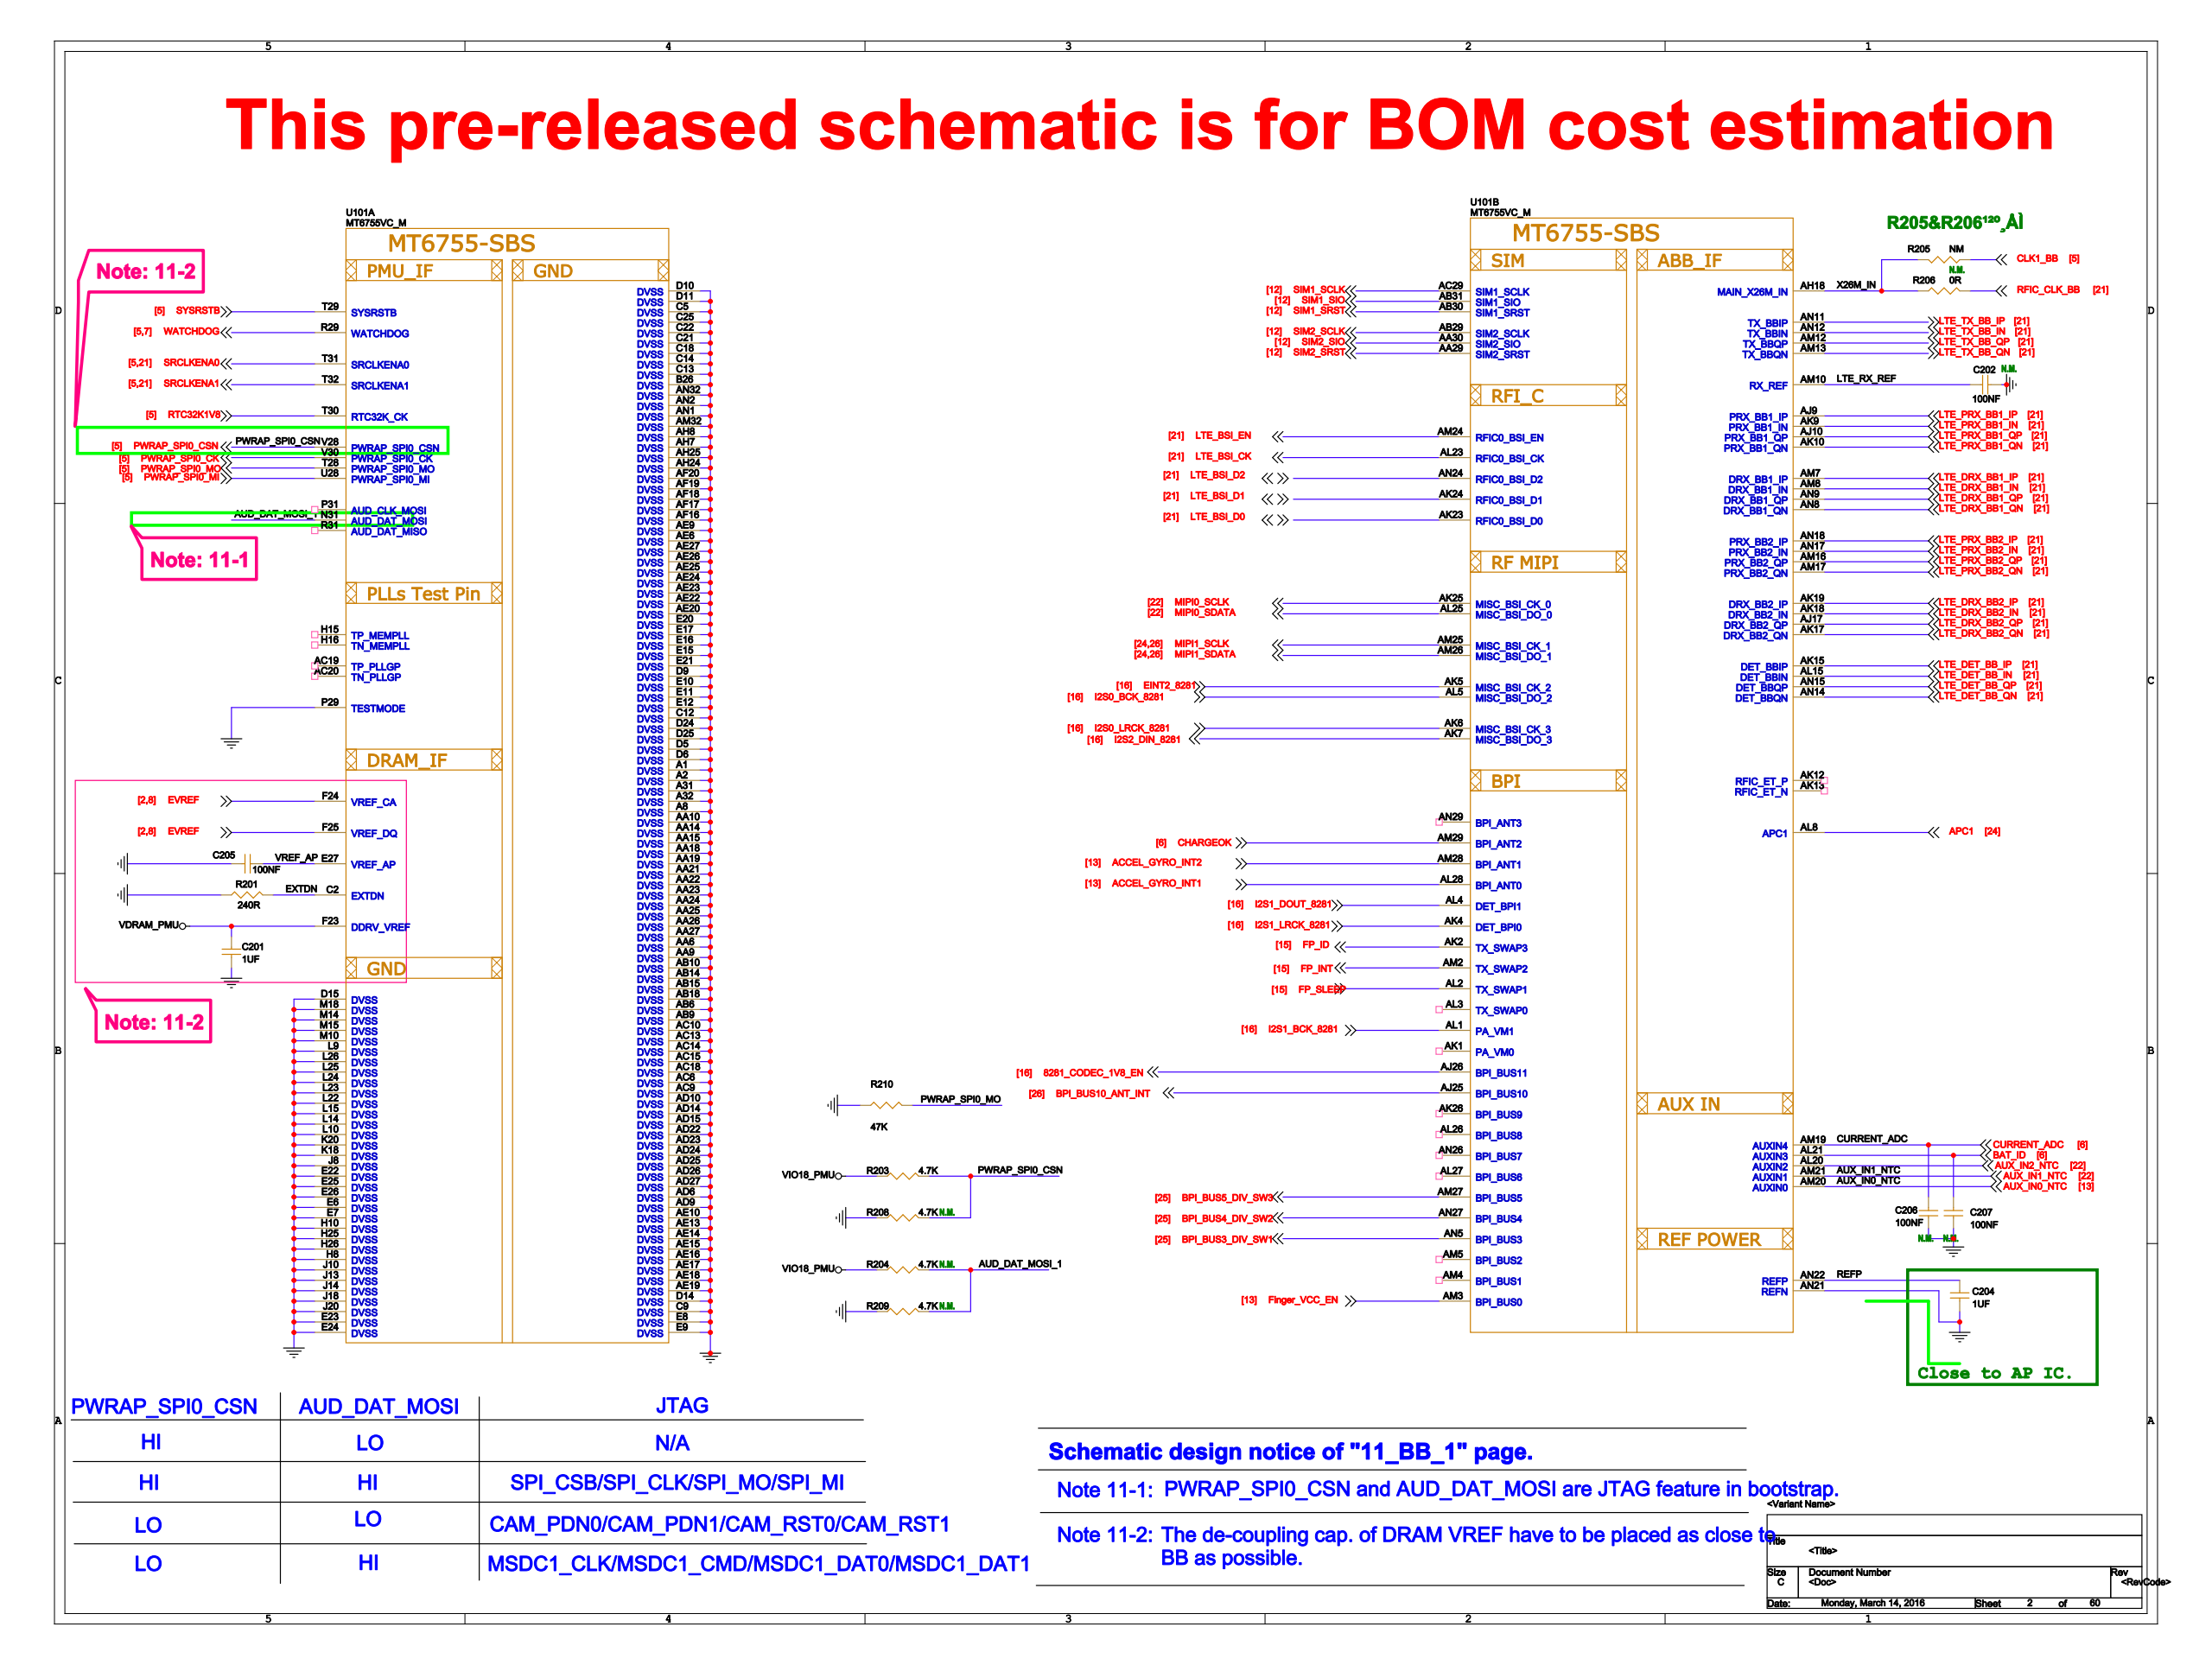Circuit board | Cadence Allegro | 1088 parts | 793 nets | one sheet of the schematic
Parts on this sheet (reference | value | footprint):
C201 | 1UF | C0201
C202
C204 | 1UF | C0201
C205 | 100NF | C0201
C206
C207
R201 | 240R | R0201
R203 | 4.7K | R0201
R204
R205
R206 | 0R | R0201
R208
R209
R210 | 47K | R0201
U101 | MT6755VC_M | MT6755
Nets of these parts (net: part-pin ...):
GND: C201-2 C202-2 C204-2 C205-2 C206-1 C207-1 R201-2 R208-1 R209-1 R210-1 U101-A1 U101-A2 U101-A8 U101-A31 U101-A32 U101-AA6 U101-AA9 U101-AA10 U101-AA14 U101-AA15 U101-AA18 U101-AA19 U101-AA21 U101-AA22 U101-AA23 U101-AA24 U101-AA25 U101-AA26 U101-AA27 U101-AB6 U101-AB9 U101-AB10 U101-AB14 U101-AB15 U101-AB18 U101-AC6 U101-AC9 U101-AC10 U101-AC13 U101-AC14 U101-AC15 U101-AC18 U101-AD6 U101-AD9 U101-AD10 U101-AD14 U101-AD15 U101-AD22 U101-AD23 U101-AD24 U101-AD25 U101-AD26 U101-AD27 U101-AE6 U101-AE9 U101-AE10 U101-AE13 U101-AE14 U101-AE15 U101-AE16 U101-AE17 U101-AE18 U101-AE19 U101-AE20 U101-AE22 U101-AE23 U101-AE24 U101-AE25 U101-AE26 U101-AE27 U101-AF16 U101-AF17 U101-AF18 U101-AF19 U101-AF20 U101-AH7 U101-AH8 U101-AH24 U101-AH25 U101-AM32 U101-AN1 U101-AN2 U101-AN21 U101-AN32 U101-B26 U101-C5 U101-C9 U101-C12 U101-C13 U101-C14 U101-C18 U101-C21 U101-C22 U101-C25 U101-D5 U101-D6 U101-D9 U101-D10 U101-D11 U101-D14 U101-D15 U101-D24 U101-D25 U101-E6 U101-E7 U101-E8 U101-E9 U101-E10 U101-E11 U101-E12 U101-E15 U101-E16 U101-E17 U101-E20 U101-E21 U101-E22 U101-E23 U101-E24 U101-E25 U101-E26 U101-H8 U101-H10 U101-H25 U101-H26 U101-J8 U101-J10 U101-J13 U101-J14 U101-J18 U101-J20 U101-K18 U101-K20 U101-L9 U101-L10 U101-L14 U101-L15 U101-L22 U101-L23 U101-L24 U101-L25 U101-L26 U101-M10 U101-M14 U101-M15 U101-M18 U101-P29
MIPI1_SCLK: U101-AM25
MIPI1_SDATA: U101-AM26
BPI_BUS5_DIV_SW3: U101-AM27
BPI_BUS4_DIV_SW2: U101-AN27
BPI_BUS3_DIV_SW1: U101-AN5
AUD_DAT_MOSI_1: R204-2 R209-2 U101-N31
VDRAM_PMU: C201-1 U101-F23
EXTDN: R201-1 U101-C2
PWRAP_SPI0_CK: U101-V30
PWRAP_SPI0_CSN: R203-2 R208-2 U101-V28
PWRAP_SPI0_MI: U101-U28
PWRAP_SPI0_MO: R210-2 U101-T28
RTC32K1V8: U101-T30
SRCLKENA0: U101-T31
SRCLKENA1: U101-T32
SYSRSTB: U101-T29
VREF_AP: C205-1 U101-E27
EVREF: U101-F24 U101-F25
WATCHDOG: U101-R29
APC1: U101-AL8
AUX_IN0_NTC: U101-AM20
AUX_IN1_NTC: U101-AM21
AUX_IN2_NTC: U101-AL20
BAT_ID: C207-2 U101-AL21
CURRENT_ADC: C206-2 U101-AM19
ACCEL_GYRO_INT1: U101-AL28
ACCEL_GYRO_INT2: U101-AM28
CHARGEOK: U101-AM29
BPI_BUS10_ANT_INT: U101-AJ25
8281_CODEC_1V8_EN: U101-AJ26
LTE_DET_BB_IN: U101-AL15
LTE_DET_BB_IP: U101-AK15
LTE_DET_BB_QN: U101-AN14
LTE_DET_BB_QP: U101-AN15
I2S1_LRCK_8281: U101-AK4
I2S1_DOUT_8281: U101-AL4
LTE_DRX_BB1_IN: U101-AM8
LTE_DRX_BB1_IP: U101-AM7
LTE_DRX_BB1_QN: U101-AN8
LTE_DRX_BB1_QP: U101-AN9
LTE_DRX_BB2_IN: U101-AK18
LTE_DRX_BB2_IP: U101-AK19
LTE_DRX_BB2_QN: U101-AK17
LTE_DRX_BB2_QP: U101-AJ17
X26M_IN: R205-2 R206-2 U101-AH18
MIPI0_SCLK: U101-AK25
EINT2_8281: U101-AK5
I2S0_LRCK_8281: U101-AK6
MIPI0_SDATA: U101-AL25
I2S0_BCK_8281: U101-AL5
I2S2_DIN_8281: U101-AK7
I2S1_BCK_8281: U101-AL1
LTE_PRX_BB1_IN: U101-AK9
LTE_PRX_BB1_IP: U101-AJ9
LTE_PRX_BB1_QN: U101-AK10
LTE_PRX_BB1_QP: U101-AJ10
LTE_PRX_BB2_IN: U101-AN17
LTE_PRX_BB2_IP: U101-AN18
LTE_PRX_BB2_QN: U101-AM17
LTE_PRX_BB2_QP: U101-AM16
REFP: C204-1 U101-AN22
LTE_BSI_CK: U101-AL23
LTE_BSI_D0: U101-AK23
LTE_BSI_D1: U101-AK24
LTE_BSI_D2: U101-AN24
LTE_BSI_EN: U101-AM24
LTE_RX_REF: C202-1 U101-AM10
SIM1_SCLK: U101-AC29
SIM1_SIO: U101-AB31
SIM1_SRST: U101-AB30
SIM2_SCLK: U101-AB29
SIM2_SIO: U101-AA30
SIM2_SRST: U101-AA29
LTE_TX_BB_IN: U101-AN12
LTE_TX_BB_IP: U101-AN11
LTE_TX_BB_QN: U101-AM13
LTE_TX_BB_QP: U101-AM12
FP_SLEEP: U101-AL2
FP_INT: U101-AM2
FP_ID: U101-AK2
VIO18_PMU: R203-1 R204-1
CLK1_BB: R205-1
RFIC_CLK_BB: R206-1